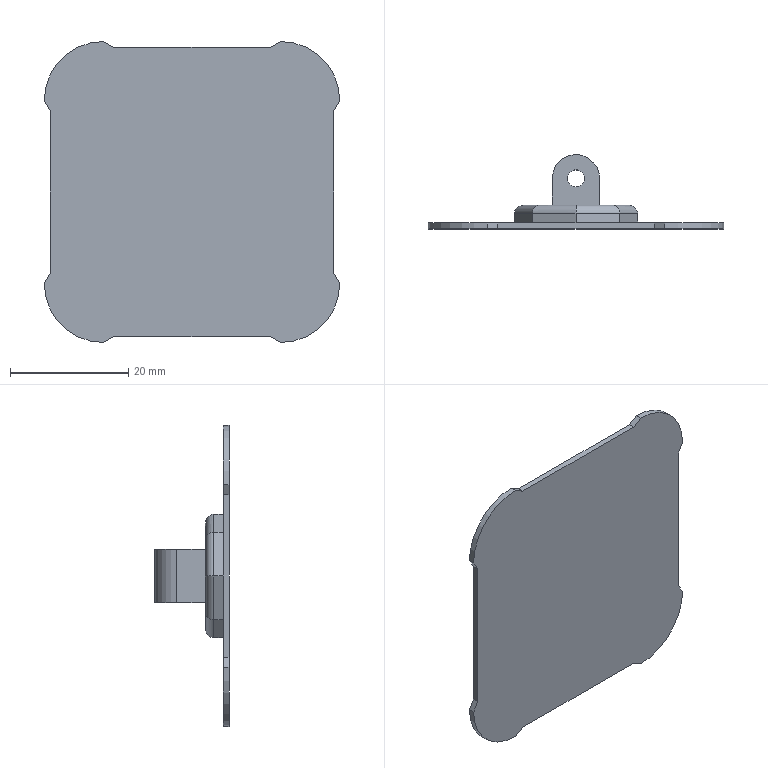Part | SolidWorks | features ICE 2, Extrusion 1, Fillet 1 | 1 solid | 42 faces | box 50 x 12.569 x 50.924 mm | volume 3739 mm3 | plane 27 | cylinder 15 | commonest cylinder face diameters 2.8 x8 20 x4 2.853 x2 8 x1
STEP:
#1=CARTESIAN_POINT('',(-1.426,8.569,4.5));
#2=VERTEX_POINT('',#1);
#3=CARTESIAN_POINT('',(1.426,8.569,4.5));
#4=VERTEX_POINT('',#3);
#5=CARTESIAN_POINT('',(0.,8.569,4.5));
#6=DIRECTION('',(0.,0.,1.));
#7=DIRECTION('',(1.,0.,0.));
#8=AXIS2_PLACEMENT_3D('',#5,#6,#7);
#9=CIRCLE('',#8,1.426);
#10=EDGE_CURVE('',#2,#4,#9,.T.);
#11=ORIENTED_EDGE('',*,*,#10,.T.);
#12=CARTESIAN_POINT('',(1.426,8.569,-4.5));
#13=VERTEX_POINT('',#12);
#14=CARTESIAN_POINT('',(1.426,8.569,4.5));
#15=DIRECTION('',(0.,0.,-1.));
#16=VECTOR('',#15,1000.);
#17=LINE('',#14,#16);
#18=EDGE_CURVE('',#4,#13,#17,.T.);
#19=ORIENTED_EDGE('',*,*,#18,.T.);
#20=CARTESIAN_POINT('',(-1.426,8.569,-4.5));
#21=VERTEX_POINT('',#20);
#22=CARTESIAN_POINT('',(0.,8.569,-4.5));
#23=DIRECTION('',(0.,0.,1.));
#24=DIRECTION('',(1.,0.,0.));
#25=AXIS2_PLACEMENT_3D('',#22,#23,#24);
#26=CIRCLE('',#25,1.426);
#27=EDGE_CURVE('',#21,#13,#26,.T.);
#28=ORIENTED_EDGE('',*,*,#27,.F.);
#29=CARTESIAN_POINT('',(-1.426,8.569,4.5));
#30=DIRECTION('',(0.,0.,-1.));
#31=VECTOR('',#30,1000.);
#32=LINE('',#29,#31);
#33=EDGE_CURVE('',#2,#21,#32,.T.);
#34=ORIENTED_EDGE('',*,*,#33,.F.);
#35=EDGE_LOOP('',(#11,#19,#28,#34));
#36=FACE_OUTER_BOUND('',#35,.T.);
#37=CARTESIAN_POINT('',(0.,8.569,4.5));
#38=DIRECTION('',(0.,0.,-1.));
#39=DIRECTION('',(-1.,0.,0.));
#40=AXIS2_PLACEMENT_3D('',#37,#38,#39);
#41=CYLINDRICAL_SURFACE('',#40,1.426);
#42=ADVANCED_FACE('',(#36),#41,.F.);
#43=CARTESIAN_POINT('',(-13.268,0.,-24.462));
#44=VERTEX_POINT('',#43);
#45=CARTESIAN_POINT('',(13.268,0.,-24.462));
#46=VERTEX_POINT('',#45);
#47=CARTESIAN_POINT('',(0.,0.,-24.462));
#48=DIRECTION('',(1.,0.,0.));
#49=VECTOR('',#48,1000.);
#50=LINE('',#47,#49);
#51=EDGE_CURVE('',#44,#46,#50,.T.);
#52=ORIENTED_EDGE('',*,*,#51,.F.);
#53=CARTESIAN_POINT('',(-13.268,1.,-24.462));
#54=VERTEX_POINT('',#53);
#55=CARTESIAN_POINT('',(-13.268,1.,-24.462));
#56=DIRECTION('',(0.,-1.,0.));
#57=VECTOR('',#56,1000.);
#58=LINE('',#55,#57);
#59=EDGE_CURVE('',#54,#44,#58,.T.);
#60=ORIENTED_EDGE('',*,*,#59,.F.);
#61=CARTESIAN_POINT('',(13.268,1.,-24.462));
#62=VERTEX_POINT('',#61);
#63=CARTESIAN_POINT('',(0.,1.,-24.462));
#64=DIRECTION('',(1.,0.,0.));
#65=VECTOR('',#64,1000.);
#66=LINE('',#63,#65);
#67=EDGE_CURVE('',#54,#62,#66,.T.);
#68=ORIENTED_EDGE('',*,*,#67,.T.);
#69=CARTESIAN_POINT('',(13.268,1.,-24.462));
#70=DIRECTION('',(0.,-1.,0.));
#71=VECTOR('',#70,1000.);
#72=LINE('',#69,#71);
#73=EDGE_CURVE('',#62,#46,#72,.T.);
#74=ORIENTED_EDGE('',*,*,#73,.T.);
#75=EDGE_LOOP('',(#52,#60,#68,#74));
#76=FACE_OUTER_BOUND('',#75,.T.);
#77=CARTESIAN_POINT('',(0.,1.,-24.462));
#78=DIRECTION('',(0.,0.,-1.));
#79=DIRECTION('',(-1.,0.,0.));
#80=AXIS2_PLACEMENT_3D('',#77,#78,#79);
#81=PLANE('',#80);
#82=ADVANCED_FACE('',(#76),#81,.T.);
#83=CARTESIAN_POINT('',(-15.,0.,-25.462));
#84=VERTEX_POINT('',#83);
#85=CARTESIAN_POINT('',(7.275,0.,-12.601));
#86=DIRECTION('',(0.866,0.,0.5));
#87=VECTOR('',#86,1000.);
#88=LINE('',#85,#87);
#89=EDGE_CURVE('',#84,#44,#88,.T.);
#90=ORIENTED_EDGE('',*,*,#89,.F.);
#91=CARTESIAN_POINT('',(-15.,1.,-25.462));
#92=VERTEX_POINT('',#91);
#93=CARTESIAN_POINT('',(-15.,1.,-25.462));
#94=DIRECTION('',(0.,-1.,0.));
#95=VECTOR('',#94,1000.);
#96=LINE('',#93,#95);
#97=EDGE_CURVE('',#92,#84,#96,.T.);
#98=ORIENTED_EDGE('',*,*,#97,.F.);
#99=CARTESIAN_POINT('',(7.275,1.,-12.601));
#100=DIRECTION('',(0.866,0.,0.5));
#101=VECTOR('',#100,1000.);
#102=LINE('',#99,#101);
#103=EDGE_CURVE('',#92,#54,#102,.T.);
#104=ORIENTED_EDGE('',*,*,#103,.T.);
#105=ORIENTED_EDGE('',*,*,#59,.T.);
#106=EDGE_LOOP('',(#90,#98,#104,#105));
#107=FACE_OUTER_BOUND('',#106,.T.);
#108=CARTESIAN_POINT('',(7.275,1.,-12.601));
#109=DIRECTION('',(0.5,0.,-0.866));
#110=DIRECTION('',(-0.866,0.,-0.5));
#111=AXIS2_PLACEMENT_3D('',#108,#109,#110);
#112=PLANE('',#111);
#113=ADVANCED_FACE('',(#107),#112,.T.);
#114=CARTESIAN_POINT('',(-25.,0.,-15.462));
#115=VERTEX_POINT('',#114);
#116=CARTESIAN_POINT('',(-15.,0.,-15.462));
#117=DIRECTION('',(0.,-1.,0.));
#118=DIRECTION('',(0.,0.,1.));
#119=AXIS2_PLACEMENT_3D('',#116,#117,#118);
#120=CIRCLE('',#119,10.);
#121=EDGE_CURVE('',#115,#84,#120,.T.);
#122=ORIENTED_EDGE('',*,*,#121,.F.);
#123=CARTESIAN_POINT('',(-25.,1.,-15.462));
#124=VERTEX_POINT('',#123);
#125=CARTESIAN_POINT('',(-25.,1.,-15.462));
#126=DIRECTION('',(0.,-1.,0.));
#127=VECTOR('',#126,1000.);
#128=LINE('',#125,#127);
#129=EDGE_CURVE('',#124,#115,#128,.T.);
#130=ORIENTED_EDGE('',*,*,#129,.F.);
#131=CARTESIAN_POINT('',(-15.,1.,-15.462));
#132=DIRECTION('',(0.,-1.,0.));
#133=DIRECTION('',(0.,0.,1.));
#134=AXIS2_PLACEMENT_3D('',#131,#132,#133);
#135=CIRCLE('',#134,10.);
#136=EDGE_CURVE('',#124,#92,#135,.T.);
#137=ORIENTED_EDGE('',*,*,#136,.T.);
#138=ORIENTED_EDGE('',*,*,#97,.T.);
#139=EDGE_LOOP('',(#122,#130,#137,#138));
#140=FACE_OUTER_BOUND('',#139,.T.);
#141=CARTESIAN_POINT('',(-15.,1.,-15.462));
#142=DIRECTION('',(0.,-1.,0.));
#143=DIRECTION('',(0.,0.,-1.));
#144=AXIS2_PLACEMENT_3D('',#141,#142,#143);
#145=CYLINDRICAL_SURFACE('',#144,10.);
#146=ADVANCED_FACE('',(#140),#145,.T.);
#147=CARTESIAN_POINT('',(-24.,0.,-13.73));
#148=VERTEX_POINT('',#147);
#149=CARTESIAN_POINT('',(-12.055,0.,6.96));
#150=DIRECTION('',(0.5,0.,0.866));
#151=VECTOR('',#150,1000.);
#152=LINE('',#149,#151);
#153=EDGE_CURVE('',#115,#148,#152,.T.);
#154=ORIENTED_EDGE('',*,*,#153,.T.);
#155=CARTESIAN_POINT('',(-24.,1.,-13.73));
#156=VERTEX_POINT('',#155);
#157=CARTESIAN_POINT('',(-24.,1.,-13.73));
#158=DIRECTION('',(0.,-1.,0.));
#159=VECTOR('',#158,1000.);
#160=LINE('',#157,#159);
#161=EDGE_CURVE('',#156,#148,#160,.T.);
#162=ORIENTED_EDGE('',*,*,#161,.F.);
#163=CARTESIAN_POINT('',(-12.055,1.,6.96));
#164=DIRECTION('',(0.5,0.,0.866));
#165=VECTOR('',#164,1000.);
#166=LINE('',#163,#165);
#167=EDGE_CURVE('',#124,#156,#166,.T.);
#168=ORIENTED_EDGE('',*,*,#167,.F.);
#169=ORIENTED_EDGE('',*,*,#129,.T.);
#170=EDGE_LOOP('',(#154,#162,#168,#169));
#171=FACE_OUTER_BOUND('',#170,.T.);
#172=CARTESIAN_POINT('',(-12.055,1.,6.96));
#173=DIRECTION('',(0.866,0.,-0.5));
#174=DIRECTION('',(-0.5,0.,-0.866));
#175=AXIS2_PLACEMENT_3D('',#172,#173,#174);
#176=PLANE('',#175);
#177=ADVANCED_FACE('',(#171),#176,.F.);
#178=CARTESIAN_POINT('',(-24.,0.,13.73));
#179=VERTEX_POINT('',#178);
#180=CARTESIAN_POINT('',(-24.,0.,0.));
#181=DIRECTION('',(0.,0.,-1.));
#182=VECTOR('',#181,1000.);
#183=LINE('',#180,#182);
#184=EDGE_CURVE('',#179,#148,#183,.T.);
#185=ORIENTED_EDGE('',*,*,#184,.F.);
#186=CARTESIAN_POINT('',(-24.,1.,13.73));
#187=VERTEX_POINT('',#186);
#188=CARTESIAN_POINT('',(-24.,1.,13.73));
#189=DIRECTION('',(0.,-1.,0.));
#190=VECTOR('',#189,1000.);
#191=LINE('',#188,#190);
#192=EDGE_CURVE('',#187,#179,#191,.T.);
#193=ORIENTED_EDGE('',*,*,#192,.F.);
#194=CARTESIAN_POINT('',(-24.,1.,0.));
#195=DIRECTION('',(0.,0.,-1.));
#196=VECTOR('',#195,1000.);
#197=LINE('',#194,#196);
#198=EDGE_CURVE('',#187,#156,#197,.T.);
#199=ORIENTED_EDGE('',*,*,#198,.T.);
#200=ORIENTED_EDGE('',*,*,#161,.T.);
#201=EDGE_LOOP('',(#185,#193,#199,#200));
#202=FACE_OUTER_BOUND('',#201,.T.);
#203=CARTESIAN_POINT('',(-24.,1.,0.));
#204=DIRECTION('',(-1.,0.,0.));
#205=DIRECTION('',(0.,0.,1.));
#206=AXIS2_PLACEMENT_3D('',#203,#204,#205);
#207=PLANE('',#206);
#208=ADVANCED_FACE('',(#202),#207,.T.);
#209=CARTESIAN_POINT('',(-25.,0.,15.462));
#210=VERTEX_POINT('',#209);
#211=CARTESIAN_POINT('',(-12.055,0.,-6.96));
#212=DIRECTION('',(0.5,0.,-0.866));
#213=VECTOR('',#212,1000.);
#214=LINE('',#211,#213);
#215=EDGE_CURVE('',#210,#179,#214,.T.);
#216=ORIENTED_EDGE('',*,*,#215,.F.);
#217=CARTESIAN_POINT('',(-25.,1.,15.462));
#218=VERTEX_POINT('',#217);
#219=CARTESIAN_POINT('',(-25.,1.,15.462));
#220=DIRECTION('',(0.,-1.,0.));
#221=VECTOR('',#220,1000.);
#222=LINE('',#219,#221);
#223=EDGE_CURVE('',#218,#210,#222,.T.);
#224=ORIENTED_EDGE('',*,*,#223,.F.);
#225=CARTESIAN_POINT('',(-12.055,1.,-6.96));
#226=DIRECTION('',(0.5,0.,-0.866));
#227=VECTOR('',#226,1000.);
#228=LINE('',#225,#227);
#229=EDGE_CURVE('',#218,#187,#228,.T.);
#230=ORIENTED_EDGE('',*,*,#229,.T.);
#231=ORIENTED_EDGE('',*,*,#192,.T.);
#232=EDGE_LOOP('',(#216,#224,#230,#231));
#233=FACE_OUTER_BOUND('',#232,.T.);
#234=CARTESIAN_POINT('',(-12.055,1.,-6.96));
#235=DIRECTION('',(-0.866,0.,-0.5));
#236=DIRECTION('',(-0.5,0.,0.866));
#237=AXIS2_PLACEMENT_3D('',#234,#235,#236);
#238=PLANE('',#237);
#239=ADVANCED_FACE('',(#233),#238,.T.);
#240=CARTESIAN_POINT('',(-15.,0.,25.462));
#241=VERTEX_POINT('',#240);
#242=CARTESIAN_POINT('',(-15.,0.,15.462));
#243=DIRECTION('',(0.,-1.,0.));
#244=DIRECTION('',(0.,0.,1.));
#245=AXIS2_PLACEMENT_3D('',#242,#243,#244);
#246=CIRCLE('',#245,10.);
#247=EDGE_CURVE('',#241,#210,#246,.T.);
#248=ORIENTED_EDGE('',*,*,#247,.F.);
#249=CARTESIAN_POINT('',(-15.,1.,25.462));
#250=VERTEX_POINT('',#249);
#251=CARTESIAN_POINT('',(-15.,1.,25.462));
#252=DIRECTION('',(0.,-1.,0.));
#253=VECTOR('',#252,1000.);
#254=LINE('',#251,#253);
#255=EDGE_CURVE('',#250,#241,#254,.T.);
#256=ORIENTED_EDGE('',*,*,#255,.F.);
#257=CARTESIAN_POINT('',(-15.,1.,15.462));
#258=DIRECTION('',(0.,-1.,0.));
#259=DIRECTION('',(0.,0.,1.));
#260=AXIS2_PLACEMENT_3D('',#257,#258,#259);
#261=CIRCLE('',#260,10.);
#262=EDGE_CURVE('',#250,#218,#261,.T.);
#263=ORIENTED_EDGE('',*,*,#262,.T.);
#264=ORIENTED_EDGE('',*,*,#223,.T.);
#265=EDGE_LOOP('',(#248,#256,#263,#264));
#266=FACE_OUTER_BOUND('',#265,.T.);
#267=CARTESIAN_POINT('',(-15.,1.,15.462));
#268=DIRECTION('',(0.,-1.,0.));
#269=DIRECTION('',(0.,0.,-1.));
#270=AXIS2_PLACEMENT_3D('',#267,#268,#269);
#271=CYLINDRICAL_SURFACE('',#270,10.);
#272=ADVANCED_FACE('',(#266),#271,.T.);
#273=CARTESIAN_POINT('',(-13.268,0.,24.462));
#274=VERTEX_POINT('',#273);
#275=CARTESIAN_POINT('',(7.275,0.,12.601));
#276=DIRECTION('',(0.866,0.,-0.5));
#277=VECTOR('',#276,1000.);
#278=LINE('',#275,#277);
#279=EDGE_CURVE('',#241,#274,#278,.T.);
#280=ORIENTED_EDGE('',*,*,#279,.T.);
#281=CARTESIAN_POINT('',(-13.268,1.,24.462));
#282=VERTEX_POINT('',#281);
#283=CARTESIAN_POINT('',(-13.268,1.,24.462));
#284=DIRECTION('',(0.,-1.,0.));
#285=VECTOR('',#284,1000.);
#286=LINE('',#283,#285);
#287=EDGE_CURVE('',#282,#274,#286,.T.);
#288=ORIENTED_EDGE('',*,*,#287,.F.);
#289=CARTESIAN_POINT('',(7.275,1.,12.601));
#290=DIRECTION('',(0.866,0.,-0.5));
#291=VECTOR('',#290,1000.);
#292=LINE('',#289,#291);
#293=EDGE_CURVE('',#250,#282,#292,.T.);
#294=ORIENTED_EDGE('',*,*,#293,.F.);
#295=ORIENTED_EDGE('',*,*,#255,.T.);
#296=EDGE_LOOP('',(#280,#288,#294,#295));
#297=FACE_OUTER_BOUND('',#296,.T.);
#298=CARTESIAN_POINT('',(7.275,1.,12.601));
#299=DIRECTION('',(-0.5,0.,-0.866));
#300=DIRECTION('',(-0.866,0.,0.5));
#301=AXIS2_PLACEMENT_3D('',#298,#299,#300);
#302=PLANE('',#301);
#303=ADVANCED_FACE('',(#297),#302,.F.);
#304=CARTESIAN_POINT('',(13.268,0.,24.462));
#305=VERTEX_POINT('',#304);
#306=CARTESIAN_POINT('',(0.,0.,24.462));
#307=DIRECTION('',(1.,0.,0.));
#308=VECTOR('',#307,1000.);
#309=LINE('',#306,#308);
#310=EDGE_CURVE('',#274,#305,#309,.T.);
#311=ORIENTED_EDGE('',*,*,#310,.T.);
#312=CARTESIAN_POINT('',(13.268,1.,24.462));
#313=VERTEX_POINT('',#312);
#314=CARTESIAN_POINT('',(13.268,1.,24.462));
#315=DIRECTION('',(0.,-1.,0.));
#316=VECTOR('',#315,1000.);
#317=LINE('',#314,#316);
#318=EDGE_CURVE('',#313,#305,#317,.T.);
#319=ORIENTED_EDGE('',*,*,#318,.F.);
#320=CARTESIAN_POINT('',(0.,1.,24.462));
#321=DIRECTION('',(1.,0.,0.));
#322=VECTOR('',#321,1000.);
#323=LINE('',#320,#322);
#324=EDGE_CURVE('',#282,#313,#323,.T.);
#325=ORIENTED_EDGE('',*,*,#324,.F.);
#326=ORIENTED_EDGE('',*,*,#287,.T.);
#327=EDGE_LOOP('',(#311,#319,#325,#326));
#328=FACE_OUTER_BOUND('',#327,.T.);
#329=CARTESIAN_POINT('',(0.,1.,24.462));
#330=DIRECTION('',(0.,0.,-1.));
#331=DIRECTION('',(-1.,0.,0.));
#332=AXIS2_PLACEMENT_3D('',#329,#330,#331);
#333=PLANE('',#332);
#334=ADVANCED_FACE('',(#328),#333,.F.);
#335=CARTESIAN_POINT('',(15.,0.,25.462));
#336=VERTEX_POINT('',#335);
#337=CARTESIAN_POINT('',(-7.275,0.,12.601));
#338=DIRECTION('',(-0.866,0.,-0.5));
#339=VECTOR('',#338,1000.);
#340=LINE('',#337,#339);
#341=EDGE_CURVE('',#336,#305,#340,.T.);
#342=ORIENTED_EDGE('',*,*,#341,.F.);
#343=CARTESIAN_POINT('',(15.,1.,25.462));
#344=VERTEX_POINT('',#343);
#345=CARTESIAN_POINT('',(15.,1.,25.462));
#346=DIRECTION('',(0.,-1.,0.));
#347=VECTOR('',#346,1000.);
#348=LINE('',#345,#347);
#349=EDGE_CURVE('',#344,#336,#348,.T.);
#350=ORIENTED_EDGE('',*,*,#349,.F.);
#351=CARTESIAN_POINT('',(-7.275,1.,12.601));
#352=DIRECTION('',(-0.866,0.,-0.5));
#353=VECTOR('',#352,1000.);
#354=LINE('',#351,#353);
#355=EDGE_CURVE('',#344,#313,#354,.T.);
#356=ORIENTED_EDGE('',*,*,#355,.T.);
#357=ORIENTED_EDGE('',*,*,#318,.T.);
#358=EDGE_LOOP('',(#342,#350,#356,#357));
#359=FACE_OUTER_BOUND('',#358,.T.);
#360=CARTESIAN_POINT('',(-7.275,1.,12.601));
#361=DIRECTION('',(-0.5,0.,0.866));
#362=DIRECTION('',(0.866,0.,0.5));
#363=AXIS2_PLACEMENT_3D('',#360,#361,#362);
#364=PLANE('',#363);
#365=ADVANCED_FACE('',(#359),#364,.T.);
#366=CARTESIAN_POINT('',(25.,0.,15.462));
#367=VERTEX_POINT('',#366);
#368=CARTESIAN_POINT('',(15.,0.,15.462));
#369=DIRECTION('',(0.,1.,0.));
#370=DIRECTION('',(0.,0.,1.));
#371=AXIS2_PLACEMENT_3D('',#368,#369,#370);
#372=CIRCLE('',#371,10.);
#373=EDGE_CURVE('',#336,#367,#372,.T.);
#374=ORIENTED_EDGE('',*,*,#373,.T.);
#375=CARTESIAN_POINT('',(25.,1.,15.462));
#376=VERTEX_POINT('',#375);
#377=CARTESIAN_POINT('',(25.,1.,15.462));
#378=DIRECTION('',(0.,-1.,0.));
#379=VECTOR('',#378,1000.);
#380=LINE('',#377,#379);
#381=EDGE_CURVE('',#376,#367,#380,.T.);
#382=ORIENTED_EDGE('',*,*,#381,.F.);
#383=CARTESIAN_POINT('',(15.,1.,15.462));
#384=DIRECTION('',(0.,1.,0.));
#385=DIRECTION('',(0.,0.,1.));
#386=AXIS2_PLACEMENT_3D('',#383,#384,#385);
#387=CIRCLE('',#386,10.);
#388=EDGE_CURVE('',#344,#376,#387,.T.);
#389=ORIENTED_EDGE('',*,*,#388,.F.);
#390=ORIENTED_EDGE('',*,*,#349,.T.);
#391=EDGE_LOOP('',(#374,#382,#389,#390));
#392=FACE_OUTER_BOUND('',#391,.T.);
#393=CARTESIAN_POINT('',(15.,1.,15.462));
#394=DIRECTION('',(0.,-1.,0.));
#395=DIRECTION('',(0.,0.,-1.));
#396=AXIS2_PLACEMENT_3D('',#393,#394,#395);
#397=CYLINDRICAL_SURFACE('',#396,10.);
#398=ADVANCED_FACE('',(#392),#397,.T.);
#399=CARTESIAN_POINT('',(24.,0.,13.73));
#400=VERTEX_POINT('',#399);
#401=CARTESIAN_POINT('',(12.055,0.,-6.96));
#402=DIRECTION('',(-0.5,0.,-0.866));
#403=VECTOR('',#402,1000.);
#404=LINE('',#401,#403);
#405=EDGE_CURVE('',#367,#400,#404,.T.);
#406=ORIENTED_EDGE('',*,*,#405,.T.);
#407=CARTESIAN_POINT('',(24.,1.,13.73));
#408=VERTEX_POINT('',#407);
#409=CARTESIAN_POINT('',(24.,1.,13.73));
#410=DIRECTION('',(0.,-1.,0.));
#411=VECTOR('',#410,1000.);
#412=LINE('',#409,#411);
#413=EDGE_CURVE('',#408,#400,#412,.T.);
#414=ORIENTED_EDGE('',*,*,#413,.F.);
#415=CARTESIAN_POINT('',(12.055,1.,-6.96));
#416=DIRECTION('',(-0.5,0.,-0.866));
#417=VECTOR('',#416,1000.);
#418=LINE('',#415,#417);
#419=EDGE_CURVE('',#376,#408,#418,.T.);
#420=ORIENTED_EDGE('',*,*,#419,.F.);
#421=ORIENTED_EDGE('',*,*,#381,.T.);
#422=EDGE_LOOP('',(#406,#414,#420,#421));
#423=FACE_OUTER_BOUND('',#422,.T.);
#424=CARTESIAN_POINT('',(12.055,1.,-6.96));
#425=DIRECTION('',(-0.866,0.,0.5));
#426=DIRECTION('',(0.5,0.,0.866));
#427=AXIS2_PLACEMENT_3D('',#424,#425,#426);
#428=PLANE('',#427);
#429=ADVANCED_FACE('',(#423),#428,.F.);
#430=CARTESIAN_POINT('',(24.,0.,-13.73));
#431=VERTEX_POINT('',#430);
#432=CARTESIAN_POINT('',(24.,0.,0.));
#433=DIRECTION('',(0.,0.,-1.));
#434=VECTOR('',#433,1000.);
#435=LINE('',#432,#434);
#436=EDGE_CURVE('',#400,#431,#435,.T.);
#437=ORIENTED_EDGE('',*,*,#436,.T.);
#438=CARTESIAN_POINT('',(24.,1.,-13.73));
#439=VERTEX_POINT('',#438);
#440=CARTESIAN_POINT('',(24.,1.,-13.73));
#441=DIRECTION('',(0.,-1.,0.));
#442=VECTOR('',#441,1000.);
#443=LINE('',#440,#442);
#444=EDGE_CURVE('',#439,#431,#443,.T.);
#445=ORIENTED_EDGE('',*,*,#444,.F.);
#446=CARTESIAN_POINT('',(24.,1.,0.));
#447=DIRECTION('',(0.,0.,-1.));
#448=VECTOR('',#447,1000.);
#449=LINE('',#446,#448);
#450=EDGE_CURVE('',#408,#439,#449,.T.);
#451=ORIENTED_EDGE('',*,*,#450,.F.);
#452=ORIENTED_EDGE('',*,*,#413,.T.);
#453=EDGE_LOOP('',(#437,#445,#451,#452));
#454=FACE_OUTER_BOUND('',#453,.T.);
#455=CARTESIAN_POINT('',(24.,1.,0.));
#456=DIRECTION('',(-1.,0.,0.));
#457=DIRECTION('',(0.,0.,1.));
#458=AXIS2_PLACEMENT_3D('',#455,#456,#457);
#459=PLANE('',#458);
#460=ADVANCED_FACE('',(#454),#459,.F.);
#461=CARTESIAN_POINT('',(25.,0.,-15.462));
#462=VERTEX_POINT('',#461);
#463=CARTESIAN_POINT('',(12.055,0.,6.96));
#464=DIRECTION('',(-0.5,0.,0.866));
#465=VECTOR('',#464,1000.);
#466=LINE('',#463,#465);
#467=EDGE_CURVE('',#462,#431,#466,.T.);
#468=ORIENTED_EDGE('',*,*,#467,.F.);
#469=CARTESIAN_POINT('',(25.,1.,-15.462));
#470=VERTEX_POINT('',#469);
#471=CARTESIAN_POINT('',(25.,1.,-15.462));
#472=DIRECTION('',(0.,-1.,0.));
#473=VECTOR('',#472,1000.);
#474=LINE('',#471,#473);
#475=EDGE_CURVE('',#470,#462,#474,.T.);
#476=ORIENTED_EDGE('',*,*,#475,.F.);
#477=CARTESIAN_POINT('',(12.055,1.,6.96));
#478=DIRECTION('',(-0.5,0.,0.866));
#479=VECTOR('',#478,1000.);
#480=LINE('',#477,#479);
#481=EDGE_CURVE('',#470,#439,#480,.T.);
#482=ORIENTED_EDGE('',*,*,#481,.T.);
#483=ORIENTED_EDGE('',*,*,#444,.T.);
#484=EDGE_LOOP('',(#468,#476,#482,#483));
#485=FACE_OUTER_BOUND('',#484,.T.);
#486=CARTESIAN_POINT('',(12.055,1.,6.96));
#487=DIRECTION('',(0.866,0.,0.5));
#488=DIRECTION('',(0.5,0.,-0.866));
#489=AXIS2_PLACEMENT_3D('',#486,#487,#488);
#490=PLANE('',#489);
#491=ADVANCED_FACE('',(#485),#490,.T.);
#492=CARTESIAN_POINT('',(15.,0.,-25.462));
#493=VERTEX_POINT('',#492);
#494=CARTESIAN_POINT('',(15.,0.,-15.462));
#495=DIRECTION('',(0.,-1.,0.));
#496=DIRECTION('',(0.,0.,1.));
#497=AXIS2_PLACEMENT_3D('',#494,#495,#496);
#498=CIRCLE('',#497,10.);
#499=EDGE_CURVE('',#493,#462,#498,.T.);
#500=ORIENTED_EDGE('',*,*,#499,.F.);
#501=CARTESIAN_POINT('',(15.,1.,-25.462));
#502=VERTEX_POINT('',#501);
#503=CARTESIAN_POINT('',(15.,1.,-25.462));
#504=DIRECTION('',(0.,-1.,0.));
#505=VECTOR('',#504,1000.);
#506=LINE('',#503,#505);
#507=EDGE_CURVE('',#502,#493,#506,.T.);
#508=ORIENTED_EDGE('',*,*,#507,.F.);
#509=CARTESIAN_POINT('',(15.,1.,-15.462));
#510=DIRECTION('',(0.,-1.,0.));
#511=DIRECTION('',(0.,0.,1.));
#512=AXIS2_PLACEMENT_3D('',#509,#510,#511);
#513=CIRCLE('',#512,10.);
#514=EDGE_CURVE('',#502,#470,#513,.T.);
#515=ORIENTED_EDGE('',*,*,#514,.T.);
#516=ORIENTED_EDGE('',*,*,#475,.T.);
#517=EDGE_LOOP('',(#500,#508,#515,#516));
#518=FACE_OUTER_BOUND('',#517,.T.);
#519=CARTESIAN_POINT('',(15.,1.,-15.462));
#520=DIRECTION('',(0.,-1.,0.));
#521=DIRECTION('',(0.,0.,-1.));
#522=AXIS2_PLACEMENT_3D('',#519,#520,#521);
#523=CYLINDRICAL_SURFACE('',#522,10.);
#524=ADVANCED_FACE('',(#518),#523,.T.);
#525=CARTESIAN_POINT('',(-7.275,0.,-12.601));
#526=DIRECTION('',(-0.866,0.,0.5));
#527=VECTOR('',#526,1000.);
#528=LINE('',#525,#527);
#529=EDGE_CURVE('',#493,#46,#528,.T.);
#530=ORIENTED_EDGE('',*,*,#529,.T.);
#531=ORIENTED_EDGE('',*,*,#73,.F.);
#532=CARTESIAN_POINT('',(-7.275,1.,-12.601));
#533=DIRECTION('',(-0.866,0.,0.5));
#534=VECTOR('',#533,1000.);
#535=LINE('',#532,#534);
#536=EDGE_CURVE('',#502,#62,#535,.T.);
#537=ORIENTED_EDGE('',*,*,#536,.F.);
#538=ORIENTED_EDGE('',*,*,#507,.T.);
#539=EDGE_LOOP('',(#530,#531,#537,#538));
#540=FACE_OUTER_BOUND('',#539,.T.);
#541=CARTESIAN_POINT('',(-7.275,1.,-12.601));
#542=DIRECTION('',(0.5,0.,0.866));
#543=DIRECTION('',(0.866,0.,-0.5));
#544=AXIS2_PLACEMENT_3D('',#541,#542,#543);
#545=PLANE('',#544);
#546=ADVANCED_FACE('',(#540),#545,.F.);
#547=CARTESIAN_POINT('',(0.,1.,10.429));
#548=VERTEX_POINT('',#547);
#549=CARTESIAN_POINT('',(7.374,1.,7.374));
#550=VERTEX_POINT('',#549);
#551=CARTESIAN_POINT('',(3.687,1.,8.902));
#552=DIRECTION('',(0.9239,0.,-0.3827));
#553=VECTOR('',#552,1000.);
#554=LINE('',#551,#553);
#555=EDGE_CURVE('',#548,#550,#554,.T.);
#556=ORIENTED_EDGE('',*,*,#555,.F.);
#557=CARTESIAN_POINT('',(-7.374,1.,7.374));
#558=VERTEX_POINT('',#557);
#559=CARTESIAN_POINT('',(-3.687,1.,8.902));
#560=DIRECTION('',(0.9239,0.,0.3827));
#561=VECTOR('',#560,1000.);
#562=LINE('',#559,#561);
#563=EDGE_CURVE('',#558,#548,#562,.T.);
#564=ORIENTED_EDGE('',*,*,#563,.F.);
#565=CARTESIAN_POINT('',(-10.429,1.,0.));
#566=VERTEX_POINT('',#565);
#567=CARTESIAN_POINT('',(-8.902,1.,3.687));
#568=DIRECTION('',(0.3827,0.,0.9239));
#569=VECTOR('',#568,1000.);
#570=LINE('',#567,#569);
#571=EDGE_CURVE('',#566,#558,#570,.T.);
#572=ORIENTED_EDGE('',*,*,#571,.F.);
#573=CARTESIAN_POINT('',(-7.374,1.,-7.374));
#574=VERTEX_POINT('',#573);
#575=CARTESIAN_POINT('',(-8.902,1.,-3.687));
#576=DIRECTION('',(-0.3827,0.,0.9239));
#577=VECTOR('',#576,1000.);
#578=LINE('',#575,#577);
#579=EDGE_CURVE('',#574,#566,#578,.T.);
#580=ORIENTED_EDGE('',*,*,#579,.F.);
#581=CARTESIAN_POINT('',(0.,1.,-10.429));
#582=VERTEX_POINT('',#581);
#583=CARTESIAN_POINT('',(-3.687,1.,-8.902));
#584=DIRECTION('',(-0.9239,0.,0.3827));
#585=VECTOR('',#584,1000.);
#586=LINE('',#583,#585);
#587=EDGE_CURVE('',#582,#574,#586,.T.);
#588=ORIENTED_EDGE('',*,*,#587,.F.);
#589=CARTESIAN_POINT('',(7.374,1.,-7.374));
#590=VERTEX_POINT('',#589);
#591=CARTESIAN_POINT('',(3.687,1.,-8.902));
#592=DIRECTION('',(-0.9239,0.,-0.3827));
#593=VECTOR('',#592,1000.);
#594=LINE('',#591,#593);
#595=EDGE_CURVE('',#590,#582,#594,.T.);
#596=ORIENTED_EDGE('',*,*,#595,.F.);
#597=CARTESIAN_POINT('',(10.429,1.,0.));
#598=VERTEX_POINT('',#597);
#599=CARTESIAN_POINT('',(8.902,1.,-3.687));
#600=DIRECTION('',(-0.3827,0.,-0.9239));
#601=VECTOR('',#600,1000.);
#602=LINE('',#599,#601);
#603=EDGE_CURVE('',#598,#590,#602,.T.);
#604=ORIENTED_EDGE('',*,*,#603,.F.);
#605=CARTESIAN_POINT('',(8.902,1.,3.687));
#606=DIRECTION('',(0.3827,0.,-0.9239));
#607=VECTOR('',#606,1000.);
#608=LINE('',#605,#607);
#609=EDGE_CURVE('',#550,#598,#608,.T.);
#610=ORIENTED_EDGE('',*,*,#609,.F.);
#611=EDGE_LOOP('',(#556,#564,#572,#580,#588,#596,#604,#610));
#612=FACE_BOUND('',#611,.T.);
#613=ORIENTED_EDGE('',*,*,#67,.F.);
#614=ORIENTED_EDGE('',*,*,#103,.F.);
#615=ORIENTED_EDGE('',*,*,#136,.F.);
#616=ORIENTED_EDGE('',*,*,#167,.T.);
#617=ORIENTED_EDGE('',*,*,#198,.F.);
#618=ORIENTED_EDGE('',*,*,#229,.F.);
#619=ORIENTED_EDGE('',*,*,#262,.F.);
#620=ORIENTED_EDGE('',*,*,#293,.T.);
#621=ORIENTED_EDGE('',*,*,#324,.T.);
#622=ORIENTED_EDGE('',*,*,#355,.F.);
#623=ORIENTED_EDGE('',*,*,#388,.T.);
#624=ORIENTED_EDGE('',*,*,#419,.T.);
#625=ORIENTED_EDGE('',*,*,#450,.T.);
#626=ORIENTED_EDGE('',*,*,#481,.F.);
#627=ORIENTED_EDGE('',*,*,#514,.F.);
#628=ORIENTED_EDGE('',*,*,#536,.T.);
#629=EDGE_LOOP('',(#613,#614,#615,#616,#617,#618,#619,#620,#621,#622,#623,#624,#625,#626,#627,#628));
#630=FACE_OUTER_BOUND('',#629,.T.);
#631=CARTESIAN_POINT('',(0.,1.,0.));
#632=DIRECTION('',(0.,1.,0.));
#633=DIRECTION('',(0.,0.,1.));
#634=AXIS2_PLACEMENT_3D('',#631,#632,#633);
#635=PLANE('',#634);
#636=ADVANCED_FACE('',(#612,#630),#635,.T.);
#637=ORIENTED_EDGE('',*,*,#51,.T.);
#638=ORIENTED_EDGE('',*,*,#529,.F.);
#639=ORIENTED_EDGE('',*,*,#499,.T.);
#640=ORIENTED_EDGE('',*,*,#467,.T.);
#641=ORIENTED_EDGE('',*,*,#436,.F.);
#642=ORIENTED_EDGE('',*,*,#405,.F.);
#643=ORIENTED_EDGE('',*,*,#373,.F.);
#644=ORIENTED_EDGE('',*,*,#341,.T.);
#645=ORIENTED_EDGE('',*,*,#310,.F.);
#646=ORIENTED_EDGE('',*,*,#279,.F.);
#647=ORIENTED_EDGE('',*,*,#247,.T.);
#648=ORIENTED_EDGE('',*,*,#215,.T.);
#649=ORIENTED_EDGE('',*,*,#184,.T.);
#650=ORIENTED_EDGE('',*,*,#153,.F.);
#651=ORIENTED_EDGE('',*,*,#121,.T.);
#652=ORIENTED_EDGE('',*,*,#89,.T.);
#653=EDGE_LOOP('',(#637,#638,#639,#640,#641,#642,#643,#644,#645,#646,#647,#648,#649,#650,#651,#652));
#654=FACE_OUTER_BOUND('',#653,.T.);
#655=CARTESIAN_POINT('',(0.,0.,0.));
#656=DIRECTION('',(0.,1.,0.));
#657=DIRECTION('',(0.,0.,1.));
#658=AXIS2_PLACEMENT_3D('',#655,#656,#657);
#659=PLANE('',#658);
#660=ADVANCED_FACE('',(#654),#659,.F.);
#661=CARTESIAN_POINT('',(7.374,2.6,7.374));
#662=VERTEX_POINT('',#661);
#663=CARTESIAN_POINT('',(7.374,4.,7.374));
#664=DIRECTION('',(0.,-1.,0.));
#665=VECTOR('',#664,1000.);
#666=LINE('',#663,#665);
#667=EDGE_CURVE('',#662,#550,#666,.T.);
#668=ORIENTED_EDGE('',*,*,#667,.F.);
#669=CARTESIAN_POINT('',(0.,2.6,10.429));
#670=VERTEX_POINT('',#669);
#671=CARTESIAN_POINT('',(0.,2.6,10.429));
#672=DIRECTION('',(-0.9239,0.,0.3827));
#673=VECTOR('',#672,1000.);
#674=LINE('',#671,#673);
#675=EDGE_CURVE('',#662,#670,#674,.T.);
#676=ORIENTED_EDGE('',*,*,#675,.T.);
#677=CARTESIAN_POINT('',(0.,4.,10.429));
#678=DIRECTION('',(0.,-1.,0.));
#679=VECTOR('',#678,1000.);
#680=LINE('',#677,#679);
#681=EDGE_CURVE('',#670,#548,#680,.T.);
#682=ORIENTED_EDGE('',*,*,#681,.T.);
#683=ORIENTED_EDGE('',*,*,#555,.T.);
#684=EDGE_LOOP('',(#668,#676,#682,#683));
#685=FACE_OUTER_BOUND('',#684,.T.);
#686=CARTESIAN_POINT('',(3.687,4.,8.902));
#687=DIRECTION('',(-0.3827,0.,-0.9239));
#688=DIRECTION('',(-0.9239,0.,0.3827));
#689=AXIS2_PLACEMENT_3D('',#686,#687,#688);
#690=PLANE('',#689);
#691=ADVANCED_FACE('',(#685),#690,.F.);
#692=CARTESIAN_POINT('',(10.429,2.6,0.));
#693=VERTEX_POINT('',#692);
#694=CARTESIAN_POINT('',(10.429,4.,0.));
#695=DIRECTION('',(0.,-1.,0.));
#696=VECTOR('',#695,1000.);
#697=LINE('',#694,#696);
#698=EDGE_CURVE('',#693,#598,#697,.T.);
#699=ORIENTED_EDGE('',*,*,#698,.F.);
#700=CARTESIAN_POINT('',(7.374,2.6,7.374));
#701=DIRECTION('',(-0.3827,0.,0.9239));
#702=VECTOR('',#701,1000.);
#703=LINE('',#700,#702);
#704=EDGE_CURVE('',#693,#662,#703,.T.);
#705=ORIENTED_EDGE('',*,*,#704,.T.);
#706=ORIENTED_EDGE('',*,*,#667,.T.);
#707=ORIENTED_EDGE('',*,*,#609,.T.);
#708=EDGE_LOOP('',(#699,#705,#706,#707));
#709=FACE_OUTER_BOUND('',#708,.T.);
#710=CARTESIAN_POINT('',(8.902,4.,3.687));
#711=DIRECTION('',(-0.9239,0.,-0.3827));
#712=DIRECTION('',(-0.3827,0.,0.9239));
#713=AXIS2_PLACEMENT_3D('',#710,#711,#712);
#714=PLANE('',#713);
#715=ADVANCED_FACE('',(#709),#714,.F.);
#716=CARTESIAN_POINT('',(7.374,2.6,-7.374));
#717=VERTEX_POINT('',#716);
#718=CARTESIAN_POINT('',(7.374,4.,-7.374));
#719=DIRECTION('',(0.,-1.,0.));
#720=VECTOR('',#719,1000.);
#721=LINE('',#718,#720);
#722=EDGE_CURVE('',#717,#590,#721,.T.);
#723=ORIENTED_EDGE('',*,*,#722,.F.);
#724=CARTESIAN_POINT('',(10.429,2.6,0.));
#725=DIRECTION('',(0.3827,0.,0.9239));
#726=VECTOR('',#725,1000.);
#727=LINE('',#724,#726);
#728=EDGE_CURVE('',#717,#693,#727,.T.);
#729=ORIENTED_EDGE('',*,*,#728,.T.);
#730=ORIENTED_EDGE('',*,*,#698,.T.);
#731=ORIENTED_EDGE('',*,*,#603,.T.);
#732=EDGE_LOOP('',(#723,#729,#730,#731));
#733=FACE_OUTER_BOUND('',#732,.T.);
#734=CARTESIAN_POINT('',(8.902,4.,-3.687));
#735=DIRECTION('',(-0.9239,0.,0.3827));
#736=DIRECTION('',(0.3827,0.,0.9239));
#737=AXIS2_PLACEMENT_3D('',#734,#735,#736);
#738=PLANE('',#737);
#739=ADVANCED_FACE('',(#733),#738,.F.);
#740=CARTESIAN_POINT('',(0.,2.6,-10.429));
#741=VERTEX_POINT('',#740);
#742=CARTESIAN_POINT('',(0.,4.,-10.429));
#743=DIRECTION('',(0.,-1.,0.));
#744=VECTOR('',#743,1000.);
#745=LINE('',#742,#744);
#746=EDGE_CURVE('',#741,#582,#745,.T.);
#747=ORIENTED_EDGE('',*,*,#746,.F.);
#748=CARTESIAN_POINT('',(7.374,2.6,-7.374));
#749=DIRECTION('',(0.9239,0.,0.3827));
#750=VECTOR('',#749,1000.);
#751=LINE('',#748,#750);
#752=EDGE_CURVE('',#741,#717,#751,.T.);
#753=ORIENTED_EDGE('',*,*,#752,.T.);
#754=ORIENTED_EDGE('',*,*,#722,.T.);
#755=ORIENTED_EDGE('',*,*,#595,.T.);
#756=EDGE_LOOP('',(#747,#753,#754,#755));
#757=FACE_OUTER_BOUND('',#756,.T.);
#758=CARTESIAN_POINT('',(3.687,4.,-8.902));
#759=DIRECTION('',(-0.3827,0.,0.9239));
#760=DIRECTION('',(0.9239,0.,0.3827));
#761=AXIS2_PLACEMENT_3D('',#758,#759,#760);
#762=PLANE('',#761);
#763=ADVANCED_FACE('',(#757),#762,.F.);
#764=CARTESIAN_POINT('',(-7.374,2.6,-7.374));
#765=VERTEX_POINT('',#764);
#766=CARTESIAN_POINT('',(-7.374,4.,-7.374));
#767=DIRECTION('',(0.,-1.,0.));
#768=VECTOR('',#767,1000.);
#769=LINE('',#766,#768);
#770=EDGE_CURVE('',#765,#574,#769,.T.);
#771=ORIENTED_EDGE('',*,*,#770,.F.);
#772=CARTESIAN_POINT('',(0.,2.6,-10.429));
#773=DIRECTION('',(0.9239,0.,-0.3827));
#774=VECTOR('',#773,1000.);
#775=LINE('',#772,#774);
#776=EDGE_CURVE('',#765,#741,#775,.T.);
#777=ORIENTED_EDGE('',*,*,#776,.T.);
#778=ORIENTED_EDGE('',*,*,#746,.T.);
#779=ORIENTED_EDGE('',*,*,#587,.T.);
#780=EDGE_LOOP('',(#771,#777,#778,#779));
#781=FACE_OUTER_BOUND('',#780,.T.);
#782=CARTESIAN_POINT('',(-3.687,4.,-8.902));
#783=DIRECTION('',(0.3827,0.,0.9239));
#784=DIRECTION('',(0.9239,0.,-0.3827));
#785=AXIS2_PLACEMENT_3D('',#782,#783,#784);
#786=PLANE('',#785);
#787=ADVANCED_FACE('',(#781),#786,.F.);
#788=CARTESIAN_POINT('',(-10.429,2.6,0.));
#789=VERTEX_POINT('',#788);
#790=CARTESIAN_POINT('',(-10.429,4.,0.));
#791=DIRECTION('',(0.,-1.,0.));
#792=VECTOR('',#791,1000.);
#793=LINE('',#790,#792);
#794=EDGE_CURVE('',#789,#566,#793,.T.);
#795=ORIENTED_EDGE('',*,*,#794,.F.);
#796=CARTESIAN_POINT('',(-7.374,2.6,-7.374));
#797=DIRECTION('',(0.3827,0.,-0.9239));
#798=VECTOR('',#797,1000.);
#799=LINE('',#796,#798);
#800=EDGE_CURVE('',#789,#765,#799,.T.);
#801=ORIENTED_EDGE('',*,*,#800,.T.);
#802=ORIENTED_EDGE('',*,*,#770,.T.);
#803=ORIENTED_EDGE('',*,*,#579,.T.);
#804=EDGE_LOOP('',(#795,#801,#802,#803));
#805=FACE_OUTER_BOUND('',#804,.T.);
#806=CARTESIAN_POINT('',(-8.902,4.,-3.687));
#807=DIRECTION('',(0.9239,0.,0.3827));
#808=DIRECTION('',(0.3827,0.,-0.9239));
#809=AXIS2_PLACEMENT_3D('',#806,#807,#808);
#810=PLANE('',#809);
#811=ADVANCED_FACE('',(#805),#810,.F.);
#812=CARTESIAN_POINT('',(-7.374,2.6,7.374));
#813=VERTEX_POINT('',#812);
#814=CARTESIAN_POINT('',(-7.374,4.,7.374));
#815=DIRECTION('',(0.,-1.,0.));
#816=VECTOR('',#815,1000.);
#817=LINE('',#814,#816);
#818=EDGE_CURVE('',#813,#558,#817,.T.);
#819=ORIENTED_EDGE('',*,*,#818,.F.);
#820=CARTESIAN_POINT('',(-10.429,2.6,0.));
#821=DIRECTION('',(-0.3827,0.,-0.9239));
#822=VECTOR('',#821,1000.);
#823=LINE('',#820,#822);
#824=EDGE_CURVE('',#813,#789,#823,.T.);
#825=ORIENTED_EDGE('',*,*,#824,.T.);
#826=ORIENTED_EDGE('',*,*,#794,.T.);
#827=ORIENTED_EDGE('',*,*,#571,.T.);
#828=EDGE_LOOP('',(#819,#825,#826,#827));
#829=FACE_OUTER_BOUND('',#828,.T.);
#830=CARTESIAN_POINT('',(-8.902,4.,3.687));
#831=DIRECTION('',(0.9239,0.,-0.3827));
#832=DIRECTION('',(-0.3827,0.,-0.9239));
#833=AXIS2_PLACEMENT_3D('',#830,#831,#832);
#834=PLANE('',#833);
#835=ADVANCED_FACE('',(#829),#834,.F.);
#836=ORIENTED_EDGE('',*,*,#681,.F.);
#837=CARTESIAN_POINT('',(-7.374,2.6,7.374));
#838=DIRECTION('',(-0.9239,0.,-0.3827));
#839=VECTOR('',#838,1000.);
#840=LINE('',#837,#839);
#841=EDGE_CURVE('',#670,#813,#840,.T.);
#842=ORIENTED_EDGE('',*,*,#841,.T.);
#843=ORIENTED_EDGE('',*,*,#818,.T.);
#844=ORIENTED_EDGE('',*,*,#563,.T.);
#845=EDGE_LOOP('',(#836,#842,#843,#844));
#846=FACE_OUTER_BOUND('',#845,.T.);
#847=CARTESIAN_POINT('',(-3.687,4.,8.902));
#848=DIRECTION('',(0.3827,0.,-0.9239));
#849=DIRECTION('',(-0.9239,0.,-0.3827));
#850=AXIS2_PLACEMENT_3D('',#847,#848,#849);
#851=PLANE('',#850);
#852=ADVANCED_FACE('',(#846),#851,.F.);
#853=CARTESIAN_POINT('',(-3.986,4.,4.5));
#854=VERTEX_POINT('',#853);
#855=CARTESIAN_POINT('',(4.,4.,4.5));
#856=VERTEX_POINT('',#855);
#857=CARTESIAN_POINT('',(0.,4.,4.5));
#858=DIRECTION('',(1.,0.,0.));
#859=VECTOR('',#858,1000.);
#860=LINE('',#857,#859);
#861=EDGE_CURVE('',#854,#856,#860,.T.);
#862=ORIENTED_EDGE('',*,*,#861,.F.);
#863=CARTESIAN_POINT('',(-3.986,4.,-4.5));
#864=VERTEX_POINT('',#863);
#865=CARTESIAN_POINT('',(-3.986,4.,4.5));
#866=DIRECTION('',(0.,0.,-1.));
#867=VECTOR('',#866,1000.);
#868=LINE('',#865,#867);
#869=EDGE_CURVE('',#854,#864,#868,.T.);
#870=ORIENTED_EDGE('',*,*,#869,.T.);
#871=CARTESIAN_POINT('',(4.,4.,-4.5));
#872=VERTEX_POINT('',#871);
#873=CARTESIAN_POINT('',(0.,4.,-4.5));
#874=DIRECTION('',(1.,0.,0.));
#875=VECTOR('',#874,1000.);
#876=LINE('',#873,#875);
#877=EDGE_CURVE('',#864,#872,#876,.T.);
#878=ORIENTED_EDGE('',*,*,#877,.T.);
#879=CARTESIAN_POINT('',(4.,4.,4.5));
#880=DIRECTION('',(0.,0.,-1.));
#881=VECTOR('',#880,1000.);
#882=LINE('',#879,#881);
#883=EDGE_CURVE('',#856,#872,#882,.T.);
#884=ORIENTED_EDGE('',*,*,#883,.F.);
#885=EDGE_LOOP('',(#862,#870,#878,#884));
#886=FACE_BOUND('',#885,.T.);
#887=CARTESIAN_POINT('',(-8.914,4.,0.));
#888=VERTEX_POINT('',#887);
#889=CARTESIAN_POINT('',(-6.303,4.,6.303));
#890=VERTEX_POINT('',#889);
#891=CARTESIAN_POINT('',(-6.081,4.,6.839));
#892=DIRECTION('',(0.3827,0.,0.9239));
#893=VECTOR('',#892,1000.);
#894=LINE('',#891,#893);
#895=EDGE_CURVE('',#888,#890,#894,.T.);
#896=ORIENTED_EDGE('',*,*,#895,.T.);
#897=CARTESIAN_POINT('',(0.,4.,8.914));
#898=VERTEX_POINT('',#897);
#899=CARTESIAN_POINT('',(0.5358,4.,9.136));
#900=DIRECTION('',(0.9239,0.,0.3827));
#901=VECTOR('',#900,1000.);
#902=LINE('',#899,#901);
#903=EDGE_CURVE('',#890,#898,#902,.T.);
#904=ORIENTED_EDGE('',*,*,#903,.T.);
#905=CARTESIAN_POINT('',(6.303,4.,6.303));
#906=VERTEX_POINT('',#905);
#907=CARTESIAN_POINT('',(6.839,4.,6.081));
#908=DIRECTION('',(0.9239,0.,-0.3827));
#909=VECTOR('',#908,1000.);
#910=LINE('',#907,#909);
#911=EDGE_CURVE('',#898,#906,#910,.T.);
#912=ORIENTED_EDGE('',*,*,#911,.T.);
#913=CARTESIAN_POINT('',(8.914,4.,0.));
#914=VERTEX_POINT('',#913);
#915=CARTESIAN_POINT('',(9.136,4.,-0.5358));
#916=DIRECTION('',(0.3827,0.,-0.9239));
#917=VECTOR('',#916,1000.);
#918=LINE('',#915,#917);
#919=EDGE_CURVE('',#906,#914,#918,.T.);
#920=ORIENTED_EDGE('',*,*,#919,.T.);
#921=CARTESIAN_POINT('',(6.303,4.,-6.303));
#922=VERTEX_POINT('',#921);
#923=CARTESIAN_POINT('',(6.081,4.,-6.839));
#924=DIRECTION('',(-0.3827,0.,-0.9239));
#925=VECTOR('',#924,1000.);
#926=LINE('',#923,#925);
#927=EDGE_CURVE('',#914,#922,#926,.T.);
#928=ORIENTED_EDGE('',*,*,#927,.T.);
#929=CARTESIAN_POINT('',(0.,4.,-8.914));
#930=VERTEX_POINT('',#929);
#931=CARTESIAN_POINT('',(-0.5358,4.,-9.136));
#932=DIRECTION('',(-0.9239,0.,-0.3827));
#933=VECTOR('',#932,1000.);
#934=LINE('',#931,#933);
#935=EDGE_CURVE('',#922,#930,#934,.T.);
#936=ORIENTED_EDGE('',*,*,#935,.T.);
#937=CARTESIAN_POINT('',(-6.303,4.,-6.303));
#938=VERTEX_POINT('',#937);
#939=CARTESIAN_POINT('',(-6.839,4.,-6.081));
#940=DIRECTION('',(-0.9239,0.,0.3827));
#941=VECTOR('',#940,1000.);
#942=LINE('',#939,#941);
#943=EDGE_CURVE('',#930,#938,#942,.T.);
#944=ORIENTED_EDGE('',*,*,#943,.T.);
#945=CARTESIAN_POINT('',(-9.136,4.,0.5358));
#946=DIRECTION('',(-0.3827,0.,0.9239));
#947=VECTOR('',#946,1000.);
#948=LINE('',#945,#947);
#949=EDGE_CURVE('',#938,#888,#948,.T.);
#950=ORIENTED_EDGE('',*,*,#949,.T.);
#951=EDGE_LOOP('',(#896,#904,#912,#920,#928,#936,#944,#950));
#952=FACE_OUTER_BOUND('',#951,.T.);
#953=CARTESIAN_POINT('',(0.,4.,0.));
#954=DIRECTION('',(0.,1.,0.));
#955=DIRECTION('',(0.,0.,1.));
#956=AXIS2_PLACEMENT_3D('',#953,#954,#955);
#957=PLANE('',#956);
#958=ADVANCED_FACE('',(#886,#952),#957,.T.);
#959=CARTESIAN_POINT('',(7.374,2.6,-7.374));
#960=CARTESIAN_POINT('',(7.374,3.42,-7.374));
#961=CARTESIAN_POINT('',(6.931,4.,-6.931));
#962=CARTESIAN_POINT('',(6.303,4.,-6.303));
#963=(BOUNDED_CURVE()B_SPLINE_CURVE(3,(#959,#960,#961,#962),.UNSPECIFIED.,.F.,.T.)B_SPLINE_CURVE_WITH_KNOTS((4,4),(3.142,4.712),.UNSPECIFIED.)CURVE()GEOMETRIC_REPRESENTATION_ITEM()RATIONAL_B_SPLINE_CURVE((1.,0.8047,0.8047,1.))REPRESENTATION_ITEM(''));
#964=EDGE_CURVE('',#717,#922,#963,.T.);
#965=ORIENTED_EDGE('',*,*,#964,.F.);
#966=ORIENTED_EDGE('',*,*,#752,.F.);
#967=CARTESIAN_POINT('',(0.,4.,-8.914));
#968=CARTESIAN_POINT('',(0.,4.,-9.801));
#969=CARTESIAN_POINT('',(0.,3.42,-10.429));
#970=CARTESIAN_POINT('',(0.,2.6,-10.429));
#971=(BOUNDED_CURVE()B_SPLINE_CURVE(3,(#967,#968,#969,#970),.UNSPECIFIED.,.F.,.T.)B_SPLINE_CURVE_WITH_KNOTS((4,4),(1.571,3.142),.UNSPECIFIED.)CURVE()GEOMETRIC_REPRESENTATION_ITEM()RATIONAL_B_SPLINE_CURVE((1.,0.8047,0.8047,1.))REPRESENTATION_ITEM(''));
#972=EDGE_CURVE('',#930,#741,#971,.T.);
#973=ORIENTED_EDGE('',*,*,#972,.F.);
#974=ORIENTED_EDGE('',*,*,#935,.F.);
#975=EDGE_LOOP('',(#965,#966,#973,#974));
#976=FACE_OUTER_BOUND('',#975,.T.);
#977=CARTESIAN_POINT('',(3.151,2.6,-7.608));
#978=DIRECTION('',(0.9239,0.,0.3827));
#979=DIRECTION('',(0.3827,0.,-0.9239));
#980=AXIS2_PLACEMENT_3D('',#977,#978,#979);
#981=CYLINDRICAL_SURFACE('',#980,1.4);
#982=ADVANCED_FACE('',(#976),#981,.T.);
#983=ORIENTED_EDGE('',*,*,#972,.T.);
#984=ORIENTED_EDGE('',*,*,#776,.F.);
#985=CARTESIAN_POINT('',(-6.303,4.,-6.303));
#986=CARTESIAN_POINT('',(-6.931,4.,-6.931));
#987=CARTESIAN_POINT('',(-7.374,3.42,-7.374));
#988=CARTESIAN_POINT('',(-7.374,2.6,-7.374));
#989=(BOUNDED_CURVE()B_SPLINE_CURVE(3,(#985,#986,#987,#988),.UNSPECIFIED.,.F.,.T.)B_SPLINE_CURVE_WITH_KNOTS((4,4),(1.571,3.142),.UNSPECIFIED.)CURVE()GEOMETRIC_REPRESENTATION_ITEM()RATIONAL_B_SPLINE_CURVE((1.,0.8047,0.8047,1.))REPRESENTATION_ITEM(''));
#990=EDGE_CURVE('',#938,#765,#989,.T.);
#991=ORIENTED_EDGE('',*,*,#990,.F.);
#992=ORIENTED_EDGE('',*,*,#943,.F.);
#993=EDGE_LOOP('',(#983,#984,#991,#992));
#994=FACE_OUTER_BOUND('',#993,.T.);
#995=CARTESIAN_POINT('',(-3.151,2.6,-7.608));
#996=DIRECTION('',(0.9239,0.,-0.3827));
#997=DIRECTION('',(-0.3827,0.,-0.9239));
#998=AXIS2_PLACEMENT_3D('',#995,#996,#997);
#999=CYLINDRICAL_SURFACE('',#998,1.4);
#1000=ADVANCED_FACE('',(#994),#999,.T.);
#1001=ORIENTED_EDGE('',*,*,#964,.T.);
#1002=ORIENTED_EDGE('',*,*,#927,.F.);
#1003=CARTESIAN_POINT('',(10.429,2.6,0.));
#1004=CARTESIAN_POINT('',(10.429,3.42,0.));
#1005=CARTESIAN_POINT('',(9.801,4.,0.));
#1006=CARTESIAN_POINT('',(8.914,4.,0.));
#1007=(BOUNDED_CURVE()B_SPLINE_CURVE(3,(#1003,#1004,#1005,#1006),.UNSPECIFIED.,.F.,.T.)B_SPLINE_CURVE_WITH_KNOTS((4,4),(3.142,4.712),.UNSPECIFIED.)CURVE()GEOMETRIC_REPRESENTATION_ITEM()RATIONAL_B_SPLINE_CURVE((1.,0.8047,0.8047,1.))REPRESENTATION_ITEM(''));
#1008=EDGE_CURVE('',#693,#914,#1007,.T.);
#1009=ORIENTED_EDGE('',*,*,#1008,.F.);
#1010=ORIENTED_EDGE('',*,*,#728,.F.);
#1011=EDGE_LOOP('',(#1001,#1002,#1009,#1010));
#1012=FACE_OUTER_BOUND('',#1011,.T.);
#1013=CARTESIAN_POINT('',(7.608,2.6,-3.151));
#1014=DIRECTION('',(0.3827,0.,0.9239));
#1015=DIRECTION('',(0.9239,0.,-0.3827));
#1016=AXIS2_PLACEMENT_3D('',#1013,#1014,#1015);
#1017=CYLINDRICAL_SURFACE('',#1016,1.4);
#1018=ADVANCED_FACE('',(#1012),#1017,.T.);
#1019=ORIENTED_EDGE('',*,*,#990,.T.);
#1020=ORIENTED_EDGE('',*,*,#800,.F.);
#1021=CARTESIAN_POINT('',(-8.914,4.,0.));
#1022=CARTESIAN_POINT('',(-9.801,4.,0.));
#1023=CARTESIAN_POINT('',(-10.429,3.42,0.));
#1024=CARTESIAN_POINT('',(-10.429,2.6,0.));
#1025=(BOUNDED_CURVE()B_SPLINE_CURVE(3,(#1021,#1022,#1023,#1024),.UNSPECIFIED.,.F.,.T.)B_SPLINE_CURVE_WITH_KNOTS((4,4),(1.571,3.142),.UNSPECIFIED.)CURVE()GEOMETRIC_REPRESENTATION_ITEM()RATIONAL_B_SPLINE_CURVE((1.,0.8047,0.8047,1.))REPRESENTATION_ITEM(''));
#1026=EDGE_CURVE('',#888,#789,#1025,.T.);
#1027=ORIENTED_EDGE('',*,*,#1026,.F.);
#1028=ORIENTED_EDGE('',*,*,#949,.F.);
#1029=EDGE_LOOP('',(#1019,#1020,#1027,#1028));
#1030=FACE_OUTER_BOUND('',#1029,.T.);
#1031=CARTESIAN_POINT('',(-7.608,2.6,-3.151));
#1032=DIRECTION('',(0.3827,0.,-0.9239));
#1033=DIRECTION('',(-0.9239,0.,-0.3827));
#1034=AXIS2_PLACEMENT_3D('',#1031,#1032,#1033);
#1035=CYLINDRICAL_SURFACE('',#1034,1.4);
#1036=ADVANCED_FACE('',(#1030),#1035,.T.);
#1037=ORIENTED_EDGE('',*,*,#1008,.T.);
#1038=ORIENTED_EDGE('',*,*,#919,.F.);
#1039=CARTESIAN_POINT('',(7.374,2.6,7.374));
#1040=CARTESIAN_POINT('',(7.374,3.42,7.374));
#1041=CARTESIAN_POINT('',(6.931,4.,6.931));
#1042=CARTESIAN_POINT('',(6.303,4.,6.303));
#1043=(BOUNDED_CURVE()B_SPLINE_CURVE(3,(#1039,#1040,#1041,#1042),.UNSPECIFIED.,.F.,.F.)B_SPLINE_CURVE_WITH_KNOTS((4,4),(3.142,4.712),.UNSPECIFIED.)CURVE()GEOMETRIC_REPRESENTATION_ITEM()RATIONAL_B_SPLINE_CURVE((1.,0.8047,0.8047,1.))REPRESENTATION_ITEM(''));
#1044=EDGE_CURVE('',#662,#906,#1043,.T.);
#1045=ORIENTED_EDGE('',*,*,#1044,.F.);
#1046=ORIENTED_EDGE('',*,*,#704,.F.);
#1047=EDGE_LOOP('',(#1037,#1038,#1045,#1046));
#1048=FACE_OUTER_BOUND('',#1047,.T.);
#1049=CARTESIAN_POINT('',(7.608,2.6,3.151));
#1050=DIRECTION('',(-0.3827,0.,0.9239));
#1051=DIRECTION('',(0.9239,0.,0.3827));
#1052=AXIS2_PLACEMENT_3D('',#1049,#1050,#1051);
#1053=CYLINDRICAL_SURFACE('',#1052,1.4);
#1054=ADVANCED_FACE('',(#1048),#1053,.T.);
#1055=ORIENTED_EDGE('',*,*,#1026,.T.);
#1056=ORIENTED_EDGE('',*,*,#824,.F.);
#1057=CARTESIAN_POINT('',(-6.303,4.,6.303));
#1058=CARTESIAN_POINT('',(-6.931,4.,6.931));
#1059=CARTESIAN_POINT('',(-7.374,3.42,7.374));
#1060=CARTESIAN_POINT('',(-7.374,2.6,7.374));
#1061=(BOUNDED_CURVE()B_SPLINE_CURVE(3,(#1057,#1058,#1059,#1060),.UNSPECIFIED.,.F.,.T.)B_SPLINE_CURVE_WITH_KNOTS((4,4),(1.571,3.142),.UNSPECIFIED.)CURVE()GEOMETRIC_REPRESENTATION_ITEM()RATIONAL_B_SPLINE_CURVE((1.,0.8047,0.8047,1.))REPRESENTATION_ITEM(''));
#1062=EDGE_CURVE('',#890,#813,#1061,.T.);
#1063=ORIENTED_EDGE('',*,*,#1062,.F.);
#1064=ORIENTED_EDGE('',*,*,#895,.F.);
#1065=EDGE_LOOP('',(#1055,#1056,#1063,#1064));
#1066=FACE_OUTER_BOUND('',#1065,.T.);
#1067=CARTESIAN_POINT('',(-7.608,2.6,3.151));
#1068=DIRECTION('',(-0.3827,0.,-0.9239));
#1069=DIRECTION('',(-0.9239,0.,0.3827));
#1070=AXIS2_PLACEMENT_3D('',#1067,#1068,#1069);
#1071=CYLINDRICAL_SURFACE('',#1070,1.4);
#1072=ADVANCED_FACE('',(#1066),#1071,.T.);
#1073=ORIENTED_EDGE('',*,*,#1044,.T.);
#1074=ORIENTED_EDGE('',*,*,#911,.F.);
#1075=CARTESIAN_POINT('',(0.,2.6,10.429));
#1076=CARTESIAN_POINT('',(0.,3.42,10.429));
#1077=CARTESIAN_POINT('',(0.,4.,9.801));
#1078=CARTESIAN_POINT('',(0.,4.,8.914));
#1079=(BOUNDED_CURVE()B_SPLINE_CURVE(3,(#1075,#1076,#1077,#1078),.UNSPECIFIED.,.F.,.T.)B_SPLINE_CURVE_WITH_KNOTS((4,4),(0.,1.571),.UNSPECIFIED.)CURVE()GEOMETRIC_REPRESENTATION_ITEM()RATIONAL_B_SPLINE_CURVE((1.,0.8047,0.8047,1.))REPRESENTATION_ITEM(''));
#1080=EDGE_CURVE('',#670,#898,#1079,.T.);
#1081=ORIENTED_EDGE('',*,*,#1080,.F.);
#1082=ORIENTED_EDGE('',*,*,#675,.F.);
#1083=EDGE_LOOP('',(#1073,#1074,#1081,#1082));
#1084=FACE_OUTER_BOUND('',#1083,.T.);
#1085=CARTESIAN_POINT('',(3.151,2.6,7.608));
#1086=DIRECTION('',(-0.9239,0.,0.3827));
#1087=DIRECTION('',(0.3827,0.,0.9239));
#1088=AXIS2_PLACEMENT_3D('',#1085,#1086,#1087);
#1089=CYLINDRICAL_SURFACE('',#1088,1.4);
#1090=ADVANCED_FACE('',(#1084),#1089,.T.);
#1091=ORIENTED_EDGE('',*,*,#1062,.T.);
#1092=ORIENTED_EDGE('',*,*,#841,.F.);
#1093=ORIENTED_EDGE('',*,*,#1080,.T.);
#1094=ORIENTED_EDGE('',*,*,#903,.F.);
#1095=EDGE_LOOP('',(#1091,#1092,#1093,#1094));
#1096=FACE_OUTER_BOUND('',#1095,.T.);
#1097=CARTESIAN_POINT('',(-3.151,2.6,7.608));
#1098=DIRECTION('',(-0.9239,0.,-0.3827));
#1099=DIRECTION('',(-0.3827,0.,0.9239));
#1100=AXIS2_PLACEMENT_3D('',#1097,#1098,#1099);
#1101=CYLINDRICAL_SURFACE('',#1100,1.4);
#1102=ADVANCED_FACE('',(#1096),#1101,.T.);
#1103=CARTESIAN_POINT('',(4.,8.569,-4.5));
#1104=VERTEX_POINT('',#1103);
#1105=CARTESIAN_POINT('',(4.,0.,-4.5));
#1106=DIRECTION('',(0.,-1.,0.));
#1107=VECTOR('',#1106,1000.);
#1108=LINE('',#1105,#1107);
#1109=EDGE_CURVE('',#1104,#872,#1108,.T.);
#1110=ORIENTED_EDGE('',*,*,#1109,.F.);
#1111=CARTESIAN_POINT('',(4.,8.569,4.5));
#1112=VERTEX_POINT('',#1111);
#1113=CARTESIAN_POINT('',(4.,8.569,4.5));
#1114=DIRECTION('',(0.,0.,-1.));
#1115=VECTOR('',#1114,1000.);
#1116=LINE('',#1113,#1115);
#1117=EDGE_CURVE('',#1112,#1104,#1116,.T.);
#1118=ORIENTED_EDGE('',*,*,#1117,.F.);
#1119=CARTESIAN_POINT('',(4.,0.,4.5));
#1120=DIRECTION('',(0.,-1.,0.));
#1121=VECTOR('',#1120,1000.);
#1122=LINE('',#1119,#1121);
#1123=EDGE_CURVE('',#1112,#856,#1122,.T.);
#1124=ORIENTED_EDGE('',*,*,#1123,.T.);
#1125=ORIENTED_EDGE('',*,*,#883,.T.);
#1126=EDGE_LOOP('',(#1110,#1118,#1124,#1125));
#1127=FACE_OUTER_BOUND('',#1126,.T.);
#1128=CARTESIAN_POINT('',(4.,0.,4.5));
#1129=DIRECTION('',(1.,0.,0.));
#1130=DIRECTION('',(0.,0.,-1.));
#1131=AXIS2_PLACEMENT_3D('',#1128,#1129,#1130);
#1132=PLANE('',#1131);
#1133=ADVANCED_FACE('',(#1127),#1132,.T.);
#1134=CARTESIAN_POINT('',(-3.986,8.904,-4.5));
#1135=VERTEX_POINT('',#1134);
#1136=CARTESIAN_POINT('',(0.,8.569,-4.5));
#1137=DIRECTION('',(0.,0.,1.));
#1138=DIRECTION('',(1.,0.,0.));
#1139=AXIS2_PLACEMENT_3D('',#1136,#1137,#1138);
#1140=CIRCLE('',#1139,4.);
#1141=EDGE_CURVE('',#1104,#1135,#1140,.T.);
#1142=ORIENTED_EDGE('',*,*,#1141,.T.);
#1143=CARTESIAN_POINT('',(-3.986,8.904,4.5));
#1144=VERTEX_POINT('',#1143);
#1145=CARTESIAN_POINT('',(-3.986,8.904,4.5));
#1146=DIRECTION('',(0.,0.,-1.));
#1147=VECTOR('',#1146,1000.);
#1148=LINE('',#1145,#1147);
#1149=EDGE_CURVE('',#1144,#1135,#1148,.T.);
#1150=ORIENTED_EDGE('',*,*,#1149,.F.);
#1151=CARTESIAN_POINT('',(0.,8.569,4.5));
#1152=DIRECTION('',(0.,0.,1.));
#1153=DIRECTION('',(1.,0.,0.));
#1154=AXIS2_PLACEMENT_3D('',#1151,#1152,#1153);
#1155=CIRCLE('',#1154,4.);
#1156=EDGE_CURVE('',#1112,#1144,#1155,.T.);
#1157=ORIENTED_EDGE('',*,*,#1156,.F.);
#1158=ORIENTED_EDGE('',*,*,#1117,.T.);
#1159=EDGE_LOOP('',(#1142,#1150,#1157,#1158));
#1160=FACE_OUTER_BOUND('',#1159,.T.);
#1161=CARTESIAN_POINT('',(0.,8.569,4.5));
#1162=DIRECTION('',(0.,0.,-1.));
#1163=DIRECTION('',(-1.,0.,0.));
#1164=AXIS2_PLACEMENT_3D('',#1161,#1162,#1163);
#1165=CYLINDRICAL_SURFACE('',#1164,4.);
#1166=ADVANCED_FACE('',(#1160),#1165,.T.);
#1167=CARTESIAN_POINT('',(-3.986,0.,-4.5));
#1168=DIRECTION('',(0.,-1.,0.));
#1169=VECTOR('',#1168,1000.);
#1170=LINE('',#1167,#1169);
#1171=EDGE_CURVE('',#1135,#864,#1170,.T.);
#1172=ORIENTED_EDGE('',*,*,#1171,.T.);
#1173=ORIENTED_EDGE('',*,*,#869,.F.);
#1174=CARTESIAN_POINT('',(-3.986,0.,4.5));
#1175=DIRECTION('',(0.,-1.,0.));
#1176=VECTOR('',#1175,1000.);
#1177=LINE('',#1174,#1176);
#1178=EDGE_CURVE('',#1144,#854,#1177,.T.);
#1179=ORIENTED_EDGE('',*,*,#1178,.F.);
#1180=ORIENTED_EDGE('',*,*,#1149,.T.);
#1181=EDGE_LOOP('',(#1172,#1173,#1179,#1180));
#1182=FACE_OUTER_BOUND('',#1181,.T.);
#1183=CARTESIAN_POINT('',(-3.986,0.,4.5));
#1184=DIRECTION('',(1.,0.,0.));
#1185=DIRECTION('',(0.,0.,-1.));
#1186=AXIS2_PLACEMENT_3D('',#1183,#1184,#1185);
#1187=PLANE('',#1186);
#1188=ADVANCED_FACE('',(#1182),#1187,.F.);
#1189=ORIENTED_EDGE('',*,*,#18,.F.);
#1190=CARTESIAN_POINT('',(0.,8.569,4.5));
#1191=DIRECTION('',(0.,0.,1.));
#1192=DIRECTION('',(1.,0.,0.));
#1193=AXIS2_PLACEMENT_3D('',#1190,#1191,#1192);
#1194=CIRCLE('',#1193,1.426);
#1195=EDGE_CURVE('',#4,#2,#1194,.T.);
#1196=ORIENTED_EDGE('',*,*,#1195,.T.);
#1197=ORIENTED_EDGE('',*,*,#33,.T.);
#1198=CARTESIAN_POINT('',(0.,8.569,-4.5));
#1199=DIRECTION('',(0.,0.,1.));
#1200=DIRECTION('',(1.,0.,0.));
#1201=AXIS2_PLACEMENT_3D('',#1198,#1199,#1200);
#1202=CIRCLE('',#1201,1.426);
#1203=EDGE_CURVE('',#13,#21,#1202,.T.);
#1204=ORIENTED_EDGE('',*,*,#1203,.F.);
#1205=EDGE_LOOP('',(#1189,#1196,#1197,#1204));
#1206=FACE_OUTER_BOUND('',#1205,.T.);
#1207=CARTESIAN_POINT('',(0.,8.569,4.5));
#1208=DIRECTION('',(0.,0.,-1.));
#1209=DIRECTION('',(-1.,0.,0.));
#1210=AXIS2_PLACEMENT_3D('',#1207,#1208,#1209);
#1211=CYLINDRICAL_SURFACE('',#1210,1.426);
#1212=ADVANCED_FACE('',(#1206),#1211,.F.);
#1213=ORIENTED_EDGE('',*,*,#861,.T.);
#1214=ORIENTED_EDGE('',*,*,#1123,.F.);
#1215=ORIENTED_EDGE('',*,*,#1156,.T.);
#1216=ORIENTED_EDGE('',*,*,#1178,.T.);
#1217=EDGE_LOOP('',(#1213,#1214,#1215,#1216));
#1218=FACE_OUTER_BOUND('',#1217,.T.);
#1219=ORIENTED_EDGE('',*,*,#10,.F.);
#1220=ORIENTED_EDGE('',*,*,#1195,.F.);
#1221=EDGE_LOOP('',(#1219,#1220));
#1222=FACE_BOUND('',#1221,.T.);
#1223=CARTESIAN_POINT('',(0.,0.,4.5));
#1224=DIRECTION('',(0.,0.,1.));
#1225=DIRECTION('',(1.,0.,0.));
#1226=AXIS2_PLACEMENT_3D('',#1223,#1224,#1225);
#1227=PLANE('',#1226);
#1228=ADVANCED_FACE('',(#1218,#1222),#1227,.T.);
#1229=ORIENTED_EDGE('',*,*,#877,.F.);
#1230=ORIENTED_EDGE('',*,*,#1171,.F.);
#1231=ORIENTED_EDGE('',*,*,#1141,.F.);
#1232=ORIENTED_EDGE('',*,*,#1109,.T.);
#1233=EDGE_LOOP('',(#1229,#1230,#1231,#1232));
#1234=FACE_OUTER_BOUND('',#1233,.T.);
#1235=ORIENTED_EDGE('',*,*,#27,.T.);
#1236=ORIENTED_EDGE('',*,*,#1203,.T.);
#1237=EDGE_LOOP('',(#1235,#1236));
#1238=FACE_BOUND('',#1237,.T.);
#1239=CARTESIAN_POINT('',(0.,0.,-4.5));
#1240=DIRECTION('',(0.,0.,1.));
#1241=DIRECTION('',(1.,0.,0.));
#1242=AXIS2_PLACEMENT_3D('',#1239,#1240,#1241);
#1243=PLANE('',#1242);
#1244=ADVANCED_FACE('',(#1234,#1238),#1243,.F.);
#1245=CLOSED_SHELL('',(#42,#82,#113,#146,#177,#208,#239,#272,#303,#334,#365,#398,#429,#460,#491,#524,#546,#636,#660,#691,#715,#739,#763,#787,#811,#835,#852,#958,#982,#1000,#1018,#1036,#1054,#1072,#1090,#1102,#1133,#1166,#1188,#1212,#1228,#1244));
#1246=MANIFOLD_SOLID_BREP('',#1245);
#1247=CARTESIAN_POINT('',(0.,0.,0.));
#1248=DIRECTION('',(0.,0.,1.));
#1249=DIRECTION('',(1.,0.,0.));
#1250=AXIS2_PLACEMENT_3D('',#1247,#1248,#1249);
#1251=(LENGTH_UNIT()NAMED_UNIT(*)SI_UNIT(.MILLI.,.METRE.));
#1252=UNCERTAINTY_MEASURE_WITH_UNIT(LENGTH_MEASURE(0.00001),#1251,'','');
#1253=(NAMED_UNIT(*)PLANE_ANGLE_UNIT()SI_UNIT($,.RADIAN.));
#1254=(NAMED_UNIT(*)SI_UNIT($,.STERADIAN.)SOLID_ANGLE_UNIT());
#1255=(GEOMETRIC_REPRESENTATION_CONTEXT(3)GLOBAL_UNCERTAINTY_ASSIGNED_CONTEXT((#1252))GLOBAL_UNIT_ASSIGNED_CONTEXT((#1251,#1253,#1254))REPRESENTATION_CONTEXT('',''));
#1256=ADVANCED_BREP_SHAPE_REPRESENTATION('',(#1246,#1250),#1255);